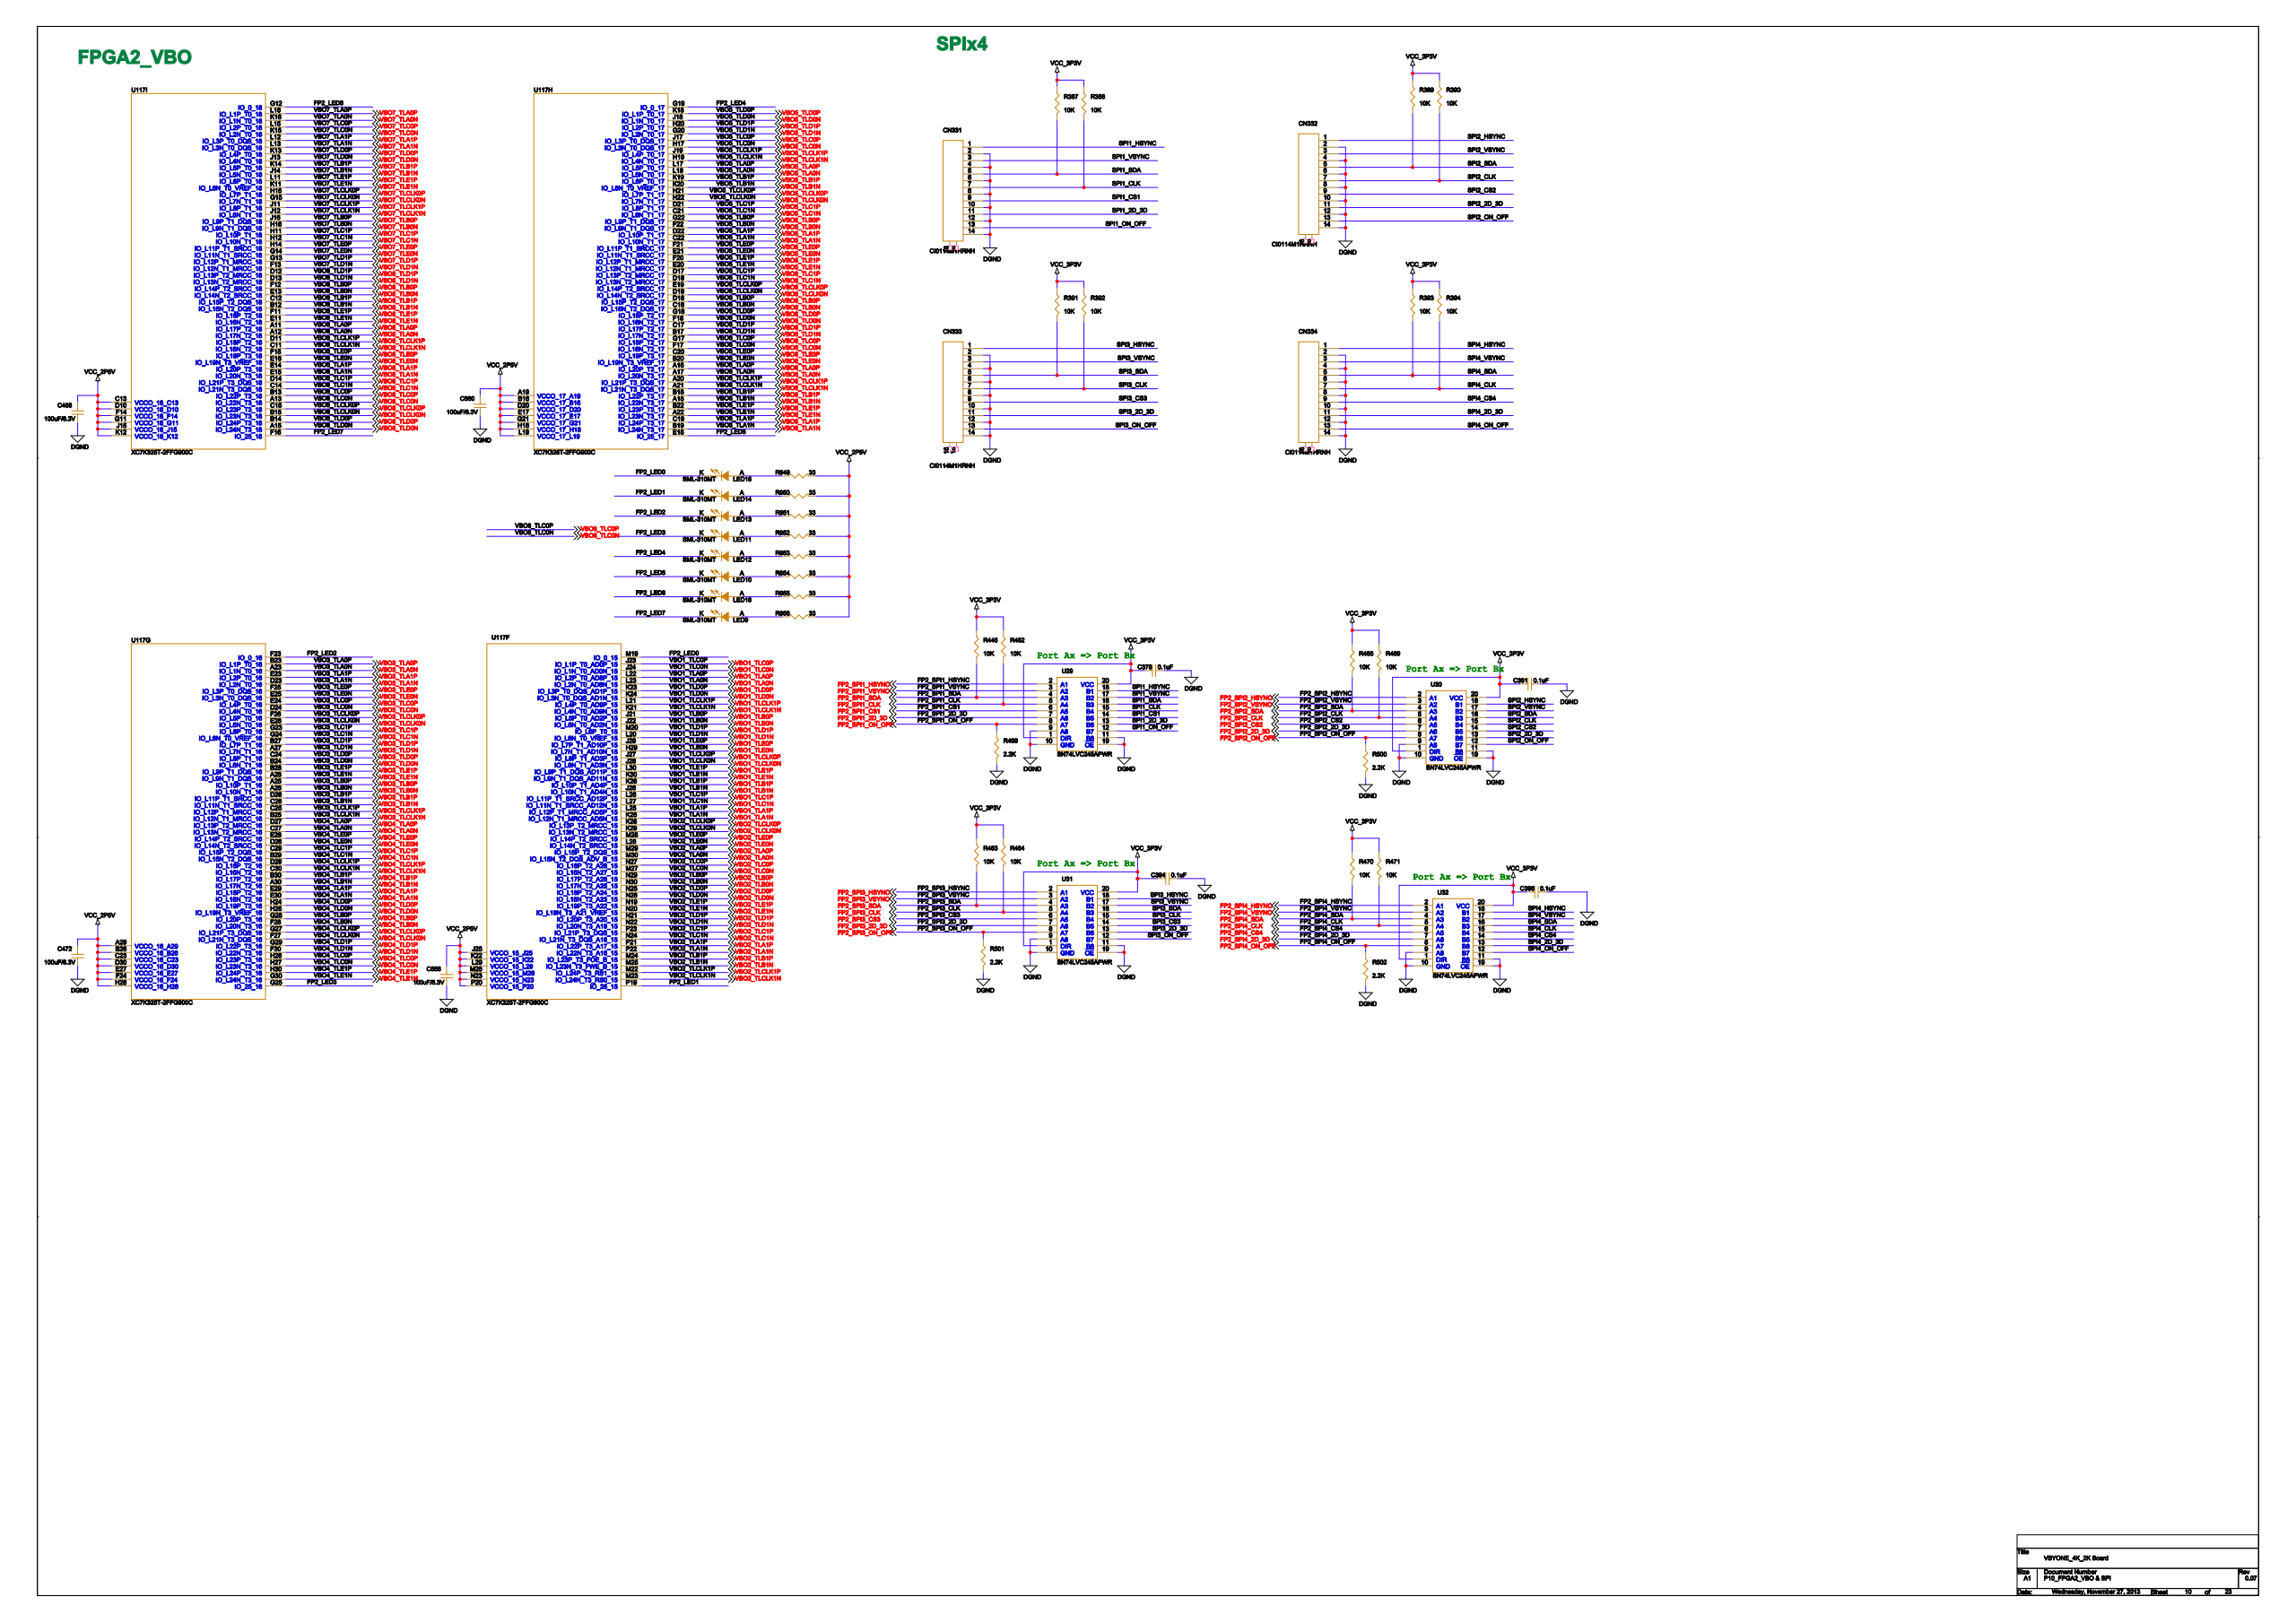Circuit board | Cadence Allegro | 1712 parts | 1495 nets | one sheet of the schematic
Parts on this sheet (reference | value | footprint):
C378 | 0.1uF | CRC1005RZAS
C381 | 0.1uF | CRC1005RZAS
C394 | 0.1uF | CRC1005RZAS
C396 | 0.1uF | CRC1005RZAS
C468 | 100uF/6.3V | CRC3225RZAS
C472 | 100uF/6.3V | CRC3225RZAS
C556 | 100uF/6.3V | CRC3225RZAS
C560 | 100uF/6.3V | CRC3225RZAS
CN331 | CI0114M1HRNH | CAC014RJAS
CN332 | CI0114M1HRNH | CAC014RJAS
CN333 | CI0114M1HRNH | CAC014RJAS
CN334 | CI0114M1HRNH | CAC014RJAS
LED9 | SML-310MT | LEC1608RZAS
LED10 | SML-310MT | LEC1608RZAS
LED11 | SML-310MT | LEC1608RZAS
LED12 | SML-310MT | LEC1608RZAS
LED13 | SML-310MT | LEC1608RZAS
LED14 | SML-310MT | LEC1608RZAS
LED15 | SML-310MT | LEC1608RZAS
LED16 | SML-310MT | LEC1608RZAS
R387 | 10K | CRC1005RZAS
R388 | 10K | CRC1005RZAS
R389 | 10K | CRC1005RZAS
R390 | 10K | CRC1005RZAS
R391 | 10K | CRC1005RZAS
R392 | 10K | CRC1005RZAS
R393 | 10K | CRC1005RZAS
R394 | 10K | CRC1005RZAS
R446 | 10K | CRC1005RZAS
R462 | 10K | CRC1005RZAS
R463 | 10K | CRC1005RZAS
R464 | 10K | CRC1005RZAS
R465 | 10K | CRC1005RZAS
R469 | 10K | CRC1005RZAS
R470 | 10K | CRC1005RZAS
R471 | 10K | CRC1005RZAS
R499 | 2.2K | CRC1005RZAS
R500 | 2.2K | CRC1005RZAS
R501 | 2.2K | CRC1005RZAS
R502 | 2.2K | CRC1005RZAS
R949 | 33 | CRC1608RZAS
R950 | 33 | CRC1608RZAS
R951 | 33 | CRC1608RZAS
R952 | 33 | CRC1608RZAS
R953 | 33 | CRC1608RZAS
R954 | 33 | CRC1608RZAS
R955 | 33 | CRC1608RZAS
R956 | 33 | CRC1608RZAS
U29 | SN74LVC245APWR | SOC020REAS
U30 | SN74LVC245APWR | SOC020REAS
U31 | SN74LVC245APWR | SOC020REAS
U32 | SN74LVC245APWR | SOC020REAS
U117 | XC7K325T-2FFG900C | BGA900RGAS
Nets of these parts (net: part-pin ...):
VCC_3P3V: C378-1 C381-1 C394-1 C396-1 R387-1 R388-1 R389-1 R390-1 R391-1 R392-1 R393-1 R394-1 R446-1 R462-1 R463-1 R464-1 R465-1 R469-1 R470-1 R471-1 U29-1 U29-20 U30-1 U30-20 U31-1 U31-20 U32-1 U32-20
DGND: C378-2 C381-2 C394-2 C396-2 C468-1 C472-1 C556-1 C560-1 CN331-2 CN331-4 CN331-6 CN331-8 CN331-10 CN331-12 CN331-14 CN332-2 CN332-4 CN332-6 CN332-8 CN332-10 CN332-12 CN332-14 CN333-2 CN333-4 CN333-6 CN333-8 CN333-10 CN333-12 CN333-14 CN334-2 CN334-4 CN334-6 CN334-8 CN334-10 CN334-12 CN334-14 R499-2 R500-2 R501-2 R502-2 U29-9 U29-10 U29-11 U29-19 U30-9 U30-10 U30-11 U30-19 U31-9 U31-10 U31-11 U31-19 U32-9 U32-10 U32-11 U32-19 U117-A1 U117-A2 U117-A5 U117-A6 U117-B4 U117-B8
VCC_2P5V: C468-2 C472-2 C556-2 C560-2 R949-2 R950-2 R951-2 R952-2 R953-2 R954-2 R955-2 R956-2 U117-A19 U117-A29 U117-B16 U117-B26 U117-C13 U117-C23 U117-D10 U117-D20 U117-D30 U117-E17 U117-E27 U117-F14 U117-F24 U117-G11 U117-G21 U117-H18 U117-H28 U117-J15 U117-J25 U117-K12 U117-K22 U117-L19 U117-L29 U117-M26 U117-N23 U117-P20
SPI1_HSYNC: CN331-1 U29-18
SPI1_VSYNC: CN331-3 U29-17
SPI1_SDA: CN331-5 R387-2 U29-16
SPI1_CLK: CN331-7 R388-2 U29-15
SPI1_CS1: CN331-9 U29-14
SPI1_2D_3D: CN331-11 U29-13
SPI1_ON_OFF: CN331-13 U29-12
SPI2_HSYNC: CN332-1 U30-18
SPI2_VSYNC: CN332-3 U30-17
SPI2_SDA: CN332-5 R389-2 U30-16
SPI2_CLK: CN332-7 R390-2 U30-15
SPI2_CS2: CN332-9 U30-14
SPI2_2D_3D: CN332-11 U30-13
SPI2_ON_OFF: CN332-13 U30-12
SPI3_HSYNC: CN333-1 U31-18
SPI3_VSYNC: CN333-3 U31-17
SPI3_SDA: CN333-5 R391-2 U31-16
SPI3_CLK: CN333-7 R392-2 U31-15
SPI3_CS3: CN333-9 U31-14
SPI3_2D_3D: CN333-11 U31-13
SPI3_ON_OFF: CN333-13 U31-12
SPI4_HSYNC: CN334-1 U32-18
SPI4_VSYNC: CN334-3 U32-17
SPI4_SDA: CN334-5 R393-2 U32-16
SPI4_CLK: CN334-7 R394-2 U32-15
SPI4_CS4: CN334-9 U32-14
SPI4_2D_3D: CN334-11 U32-13
SPI4_ON_OFF: CN334-13 U32-12
N19798786: LED10-A R954-1
FP2_LED5: LED10-K U117-E18
N19798790: LED11-A R952-1
FP2_LED3: LED11-K U117-G25
N19798788: LED12-A R953-1
FP2_LED4: LED12-K U117-G19
N19798792: LED13-A R951-1
FP2_LED2: LED13-K U117-F23
N19798794: LED14-A R950-1
FP2_LED1: LED14-K U117-P19
N19798796: LED15-A R949-1
FP2_LED0: LED15-K U117-M19
N19798784: LED16-A R955-1
FP2_LED6: LED16-K U117-G12
N19798782: LED9-A R956-1
FP2_LED7: LED9-K U117-F16
FP2_SPI1_SDA: R446-2 U29-4
FP2_SPI1_CLK: R462-2 U29-5
FP2_SPI3_SDA: R463-2 U31-4
FP2_SPI3_CLK: R464-2 U31-5
FP2_SPI2_SDA: R465-2 U30-4
FP2_SPI2_CLK: R469-2 U30-5
FP2_SPI4_SDA: R470-2 U32-4
FP2_SPI4_CLK: R471-2 U32-5
FP2_SPI1_ON_OFF: R499-1 U29-8
FP2_SPI2_ON_OFF: R500-1 U30-8
FP2_SPI3_ON_OFF: R501-1 U31-8 U117-U29
FP2_SPI4_ON_OFF: R502-1 U32-8
FP2_SPI1_HSYNC: U29-2
FP2_SPI1_VSYNC: U29-3
FP2_SPI1_CS1: U29-6
FP2_SPI1_2D_3D: U29-7
FP2_SPI2_HSYNC: U30-2
FP2_SPI2_VSYNC: U30-3
FP2_SPI2_CS2: U30-6
FP2_SPI2_2D_3D: U30-7
FP2_SPI3_HSYNC: U31-2
FP2_SPI3_VSYNC: U31-3
FP2_SPI3_CS3: U31-6
FP2_SPI3_2D_3D: U31-7 U117-U30
FP2_SPI4_HSYNC: U32-2
FP2_SPI4_VSYNC: U32-3
FP2_SPI4_CS4: U32-6
FP2_SPI4_2D_3D: U32-7
VBO7_TLE1P: U117-L11
VBO7_TLE1N: U117-K11
VBO7_TLCLK1P: U117-J11
VBO7_TLC1P: U117-H11
VBO8_TLE1P: U117-F11
VBO8_TLE1N: U117-E11
VBO8_TLCLK1P: U117-D11
VBO8_TLCLK1N: U117-C11
VBO8_TLA0P: U117-A11
VBO7_TLA1P: U117-L12
VBO7_TLCLK1N: U117-J12
VBO7_TLC1N: U117-H12
VBO8_TLB0P: U117-F12
VBO8_TLD1P: U117-D12
VBO8_TLB1P: U117-C12
VBO8_TLB1N: U117-B12
VBO8_TLA0N: U117-A12
VBO7_TLA1N: U117-L13
VBO7_TLD0P: U117-K13
VBO7_TLD0N: U117-J13
VBO7_TLD1P: U117-G13
VBO7_TLD1N: U117-F13
VBO8_TLB0N: U117-E13
VBO8_TLD1N: U117-D13
VBO8_TLC0P: U117-B13
VBO8_TLC0N: U117-A13
VBO7_TLB1P: U117-K14
VBO7_TLB1N: U117-J14
VBO7_TLE0P: U117-H14
VBO7_TLE0N: U117-G14
VBO8_TLA1P: U117-E14
VBO8_TLC1P: U117-D14
VBO8_TLC1N: U117-C14
VBO8_TLD0P: U117-B14
VBO7_TLC0P: U117-L15
VBO7_TLC0N: U117-K15
VBO7_TLCLK0P: U117-H15
VBO7_TLCLK0N: U117-G15
VBO8_TLE0P: U117-F15
VBO8_TLA1N: U117-E15
VBO8_TLCLK0P: U117-C15
VBO8_TLCLK0N: U117-B15
VBO8_TLD0N: U117-A15
VBO7_TLA0P: U117-L16
VBO7_TLA0N: U117-K16
VBO7_TLB0P: U117-J16
VBO7_TLB0N: U117-H16
VBO8_TLE0N: U117-E16
VBO6_TLB0P: U117-D16
VBO6_TLB0N: U117-C16
VBO6_TLA0P: U117-A16
VBO5_TLA0P: U117-L17
VBO5_TLC0P: U117-J17
VBO5_TLC0N: U117-H17
VBO6_TLC0P: U117-G17
VBO6_TLC0N: U117-F17
VBO6_TLC1P: U117-D17
VBO6_TLD1P: U117-C17
VBO6_TLD1N: U117-B17
VBO6_TLA0N: U117-A17
VBO5_TLA0N: U117-L18
VBO5_TLD0P: U117-K18
VBO5_TLD0N: U117-J18
VBO6_TLD0P: U117-G18
VBO6_TLD0N: U117-F18
VBO6_TLC1N: U117-D18
VBO6_TLB1P: U117-B18
VBO6_TLB1N: U117-A18
VBO2_TLE1P: U117-N19
VBO5_TLB1P: U117-K19
VBO5_TLCLK1P: U117-J19
VBO5_TLCLK1N: U117-H19
VBO6_TLCLK0P: U117-E19
VBO6_TLCLK0N: U117-D19
VBO6_TLA1P: U117-C19
VBO6_TLA1N: U117-B19
VBO2_TLE1N: U117-N20
VBO1_TLD1P: U117-M20
VBO1_TLD1N: U117-L20
VBO5_TLB1N: U117-K20
VBO5_TLD1P: U117-H20
VBO5_TLD1N: U117-G20
VBO5_TLE1P: U117-F20
VBO5_TLE1N: U117-E20
VBO6_TLE0P: U117-C20
VBO6_TLE0N: U117-B20
VBO6_TLCLK1P: U117-A20
VBO2_TLA1P: U117-P21
VBO2_TLD1P: U117-N21
VBO1_TLCLK1P: U117-L21
VBO1_TLCLK1N: U117-K21
VBO1_TLB0P: U117-J21
VBO5_TLCLK0P: U117-H21
VBO5_TLE0P: U117-F21
VBO5_TLE0N: U117-E21
VBO5_TLC1P: U117-D21
VBO5_TLC1N: U117-C21
VBO6_TLCLK1N: U117-A21
VBO2_TLA1N: U117-P22
VBO2_TLD1N: U117-N22
VBO2_TLCLK1P: U117-M22
VBO1_TLA0P: U117-L22
VBO1_TLB0N: U117-J22
VBO5_TLCLK0N: U117-H22
VBO5_TLB0P: U117-G22
VBO5_TLB0N: U117-F22
VBO5_TLA1P: U117-D22
VBO5_TLA1N: U117-C22
VBO6_TLE1P: U117-B22
VBO6_TLE1N: U117-A22
VBO2_TLC1P: U117-P23
VBO2_TLCLK1N: U117-M23
VBO1_TLA0N: U117-L23
VBO1_TLD0P: U117-K23
VBO1_TLC0P: U117-J23
VBO3_TLC1P: U117-G23
VBO3_TLA1P: U117-E23
VBO3_TLA1N: U117-D23
VBO3_TLA0P: U117-B23
VBO3_TLA0N: U117-A23
VBO2_TLC1N: U117-N24
VBO2_TLB1P: U117-M24
VBO1_TLD0N: U117-K24
VBO1_TLC0N: U117-J24
VBO4_TLD0P: U117-H24
VBO3_TLC1N: U117-G24
VBO3_TLC0P: U117-E24
VBO3_TLC0N: U117-D24
VBO3_TLD0P: U117-C24
VBO3_TLD0N: U117-B24
VBO2_TLD0P: U117-N25
VBO2_TLB1N: U117-M25
VBO1_TLA1P: U117-L25
VBO1_TLA1N: U117-K25
VBO4_TLD0N: U117-H25
VBO3_TLE0P: U117-F25
VBO3_TLE0N: U117-E25
VBO3_TLCLK1P: U117-C25
VBO3_TLCLK1N: U117-B25
VBO3_TLB0P: U117-A25
VBO2_TLD0N: U117-N26
VBO1_TLC1P: U117-L26
VBO1_TLB1P: U117-K26
VBO1_TLB1N: U117-J26
VBO4_TLC0P: U117-H26
VBO3_TLCLK0P: U117-F26
VBO3_TLCLK0N: U117-E26
VBO3_TLB1P: U117-D26
VBO3_TLB1N: U117-C26
VBO3_TLB0N: U117-A26
VBO2_TLC0P: U117-N27
VBO2_TLC0N: U117-M27
VBO1_TLC1N: U117-L27
VBO1_TLCLK0P: U117-J27
VBO4_TLC0N: U117-H27
VBO4_TLCLK0P: U117-G27
VBO4_TLCLK0N: U117-F27
VBO4_TLA0P: U117-D27
VBO4_TLA0N: U117-C27
VBO3_TLD1P: U117-B27
VBO3_TLD1N: U117-A27
VBO2_TLE0P: U117-M28
VBO2_TLE0N: U117-L28
VBO2_TLCLK0P: U117-K28
VBO1_TLCLK0N: U117-J28
VBO4_TLB0P: U117-G28
VBO4_TLB0N: U117-F28
VBO4_TLE0P: U117-E28
VBO4_TLE0N: U117-D28
VBO3_TLE1P: U117-B28
VBO3_TLE1N: U117-A28
VBO2_TLB0P: U117-N29
VBO2_TLA0P: U117-M29
VBO2_TLCLK0N: U117-K29
VBO1_TLE0P: U117-J29
VBO1_TLE0N: U117-H29
VBO4_TLD1P: U117-G29
VBO4_TLA1P: U117-E29
VBO4_TLCLK1P: U117-D29
VBO4_TLC1P: U117-C29
VBO4_TLC1N: U117-B29
VBO2_TLB0N: U117-N30
VBO2_TLA0N: U117-M30
VBO1_TLE1P: U117-L30
VBO1_TLE1N: U117-K30
VBO4_TLE1P: U117-H30
VBO4_TLE1N: U117-G30
VBO4_TLD1N: U117-F30
VBO4_TLA1N: U117-E30
VBO4_TLCLK1N: U117-C30
VBO4_TLB1P: U117-B30
VBO4_TLB1N: U117-A30